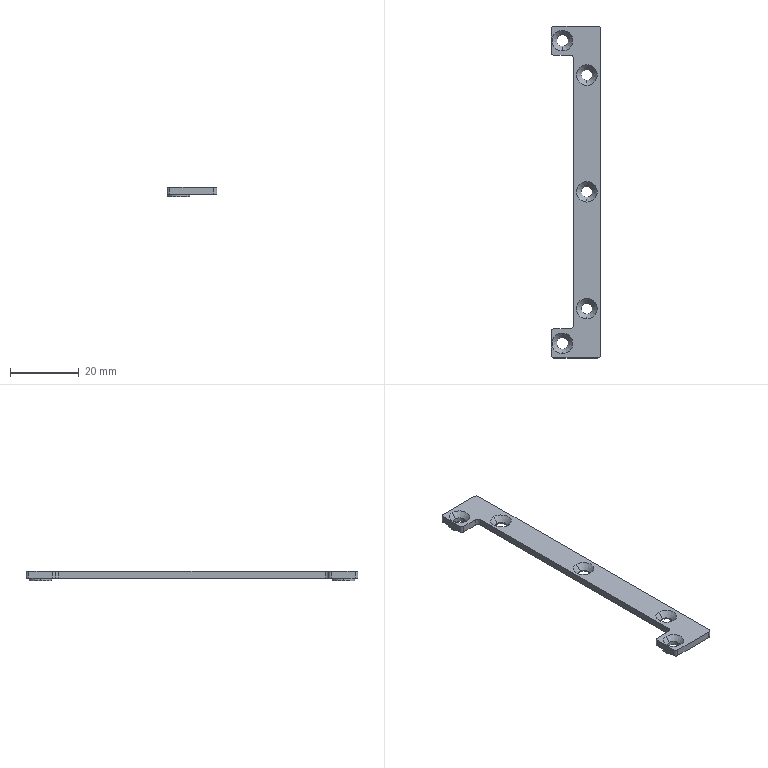NC program | NX | posted with a generic post | part box 14.52 x 96.5 x 2.7 mm
Whole program:
N10 G17 G21 G94 G90
(FLOOR_WALL , TOOL : D6)
N12 T06 M6
N14 G54
N16 G17 G0 G90 X57.25 Y-10.257 S9500 M3
N18 G43 Z30. H6
N20 Z3.
N22 G94 G1 Z0. F1500.
N24 X54.25
N26 X-54.25
N28 Y-7.669
N30 X54.25
N32 Y-5.081
N34 X-54.25
N36 Y-2.493
N38 X54.25
N40 Y0.096
N42 X-54.25
N44 Y2.684
N46 X54.25
N48 Y5.272
N50 X-54.25
N52 Y7.86
N54 X54.25
N56 X57.25
N58 Z3.
N60 G0 Z30.
N62 M5
(DRILLING , TOOL : D6A45)
N64 T07 M6
N66 G54
N68 G17 G0 G90 X-44. Y-3.96 S5000 M3
N70 G43 Z30. H7
N72 G94 G81 G98 Z-3. F250. R3.
N74 X-34. Y3.15
N76 X-0.05
N78 X33.9
N80 X44. Y-3.96
N82 G80
N84 G0 X44. Y-3.96 Z30.
N86 M5
(CAVITY_MILL , TOOL : D4)
N88 T04 M6
N90 G54
N92 G17 G0 G90 X2.078 Y-13.057 S9500 M3
N94 G43 Z30. H4
N96 Z0.614
N98 G95 G1 Z-0.386 F1.579
N100 X0.866 Y-10.957
N102 G3 X0. Y-10.457 R1.
N104 G94 G1 X-51.248 F2500.
N106 G2 X-51.448 Y-10.265 R0.205
N108 G1 Y10.265
N110 G2 X-51.248 Y10.458 R0.205
N112 G1 X51.248
N114 G2 X51.447 Y10.265 R0.205
N116 G1 Y-10.265
N118 G2 X51.248 Y-10.457 R0.204
N120 G1 X0.
N122 Y-7.657
N124 X-37.304
N126 G3 X-37.09 Y-6.46 R3.46
N128 G1 Y-3.32
N130 X37.09
N132 Y-6.46
N134 G3 X37.304 Y-7.657 R3.46
N136 G1 X37.829 Y-7.464
N138 G2 X37.65 Y-6.46 R2.9
N140 G1 Y-2.76
N142 X-37.65
N144 Y-6.46
N146 G2 X-40.55 Y-9.36 R2.9
N148 G1 X-47.45
N150 G2 X-50.35 Y-6.46 R2.9
N152 G1 Y6.26
N154 G2 X-47.25 Y9.36 R3.1
N156 G1 X47.25
N158 G2 X50.35 Y6.26 R3.1
N160 G1 Y-6.46
N162 G2 X47.45 Y-9.36 R2.9
N164 G1 X40.55
N166 G2 X37.829 Y-7.464 R2.9
N168 G1 X37.304 Y-7.657
N170 X0.
N172 Y-5.857
N174 X-35.29
N176 Y-5.12
N178 X35.29
N180 Y-5.857
N182 X0.
N184 G3 X-0.866 Y-6.357 R1.
N186 G1 Z0.614
N188 G0 Z30.
N190 X2.078 Y-13.058
N192 Z0.229
N194 G95 G1 Z-0.771 F1.579
N196 X0.866 Y-10.958
N198 G3 X0. Y-10.458 R1.
N200 G94 G1 X-51.248 F2500.
N202 G2 X-51.448 Y-10.265 R0.205
N204 G1 Y10.265
N206 G2 X-51.248 Y10.458 R0.205
N208 G1 X51.248
N210 G2 X51.447 Y10.265 R0.205
N212 G1 Y-10.265
N214 G2 X51.248 Y-10.458 R0.204
N216 G1 X0.
N218 Y-7.658
N220 X-37.304
N222 G3 X-37.09 Y-6.46 R3.46
N224 G1 Y-3.32
N226 X37.09
N228 Y-6.46
N230 G3 X37.304 Y-7.658 R3.46
N232 G1 X37.829 Y-7.464
N234 G2 X37.65 Y-6.46 R2.9
N236 G1 Y-2.76
N238 X-37.65
N240 Y-6.46
N242 G2 X-40.55 Y-9.36 R2.9
N244 G1 X-47.45
N246 G2 X-50.35 Y-6.46 R2.9
N248 G1 Y6.26
N250 G2 X-47.25 Y9.36 R3.1
N252 G1 X47.25
N254 G2 X50.35 Y6.26 R3.1
N256 G1 Y-6.46
N258 G2 X47.45 Y-9.36 R2.9
N260 G1 X40.55
N262 G2 X37.829 Y-7.464 R2.9
N264 G1 X37.304 Y-7.658
N266 X0.
N268 Y-5.858
N270 X-35.29
N272 Y-5.12
N274 X35.29
N276 Y-5.858
N278 X0.
N280 G3 X-0.866 Y-6.358 R1.
N282 G1 Z0.229
N284 G0 X2.078 Y-13.058 Z-0.157
N286 G95 G1 Z-1.157 F1.579
N288 X0.866 Y-10.958
N290 G3 X0. Y-10.458 R1.
N292 G94 G1 X-51.248 F2500.
N294 G2 X-51.448 Y-10.264 R0.205
N296 G1 Y10.265
N298 G2 X-51.248 Y10.459 R0.206
N300 G1 X51.247
N302 G2 X51.448 Y10.265 R0.205
N304 G1 Y-10.265
N306 G2 X51.248 Y-10.458 R0.205
N308 G1 X0.
N310 Y-7.658
N312 X-37.304
N314 G3 X-37.09 Y-6.46 R3.46
N316 G1 Y-3.32
N318 X37.09
N320 Y-6.46
N322 G3 X37.304 Y-7.658 R3.46
N324 G1 X37.829 Y-7.464
N326 G2 X37.65 Y-6.46 R2.9
N328 G1 Y-2.76
N330 X-37.65
N332 Y-6.46
N334 G2 X-40.55 Y-9.36 R2.9
N336 G1 X-47.45
N338 G2 X-50.35 Y-6.46 R2.9
N340 G1 Y6.26
N342 G2 X-47.25 Y9.36 R3.1
N344 G1 X47.25
N346 G2 X50.35 Y6.26 R3.1
N348 G1 Y-6.46
N350 G2 X47.45 Y-9.36 R2.9
N352 G1 X40.55
N354 G2 X37.829 Y-7.464 R2.9
N356 G1 X37.304 Y-7.658
N358 X0.
N360 Y-5.858
N362 X-35.29
N364 Y-5.12
N366 X35.29
N368 Y-5.858
N370 X0.
N372 G3 X-0.866 Y-6.358 R1.
N374 G1 Z-0.157
N376 G0 X2.078 Y-13.058 Z-0.543
N378 G95 G1 Z-1.543 F1.579
N380 X0.866 Y-10.958
N382 G3 X0. Y-10.458 R1.
N384 G94 G1 X-51.248 F2500.
N386 G2 X-51.449 Y-10.264 R0.206
N388 G1 Y10.264
N390 G2 X-51.247 Y10.459 R0.207
N392 G1 X51.247
N394 G2 X51.448 Y10.265 R0.206
N396 G1 Y-10.265
N398 G2 X51.248 Y-10.458 R0.205
N400 G1 X0.
N402 Y-7.658
N404 X-37.304
N406 G3 X-37.09 Y-6.46 R3.46
N408 G1 Y-3.32
N410 X37.09
N412 Y-6.46
N414 G3 X37.304 Y-7.658 R3.46
N416 G1 X37.829 Y-7.464
N418 G2 X37.65 Y-6.46 R2.9
N420 G1 Y-2.76
N422 X-37.65
N424 Y-6.46
N426 G2 X-40.55 Y-9.36 R2.9
N428 G1 X-47.45
N430 G2 X-50.35 Y-6.46 R2.9
N432 G1 Y6.26
N434 G2 X-47.25 Y9.36 R3.1
N436 G1 X47.25
N438 G2 X50.35 Y6.26 R3.1
N440 G1 Y-6.46
N442 G2 X47.45 Y-9.36 R2.9
N444 G1 X40.55
N446 G2 X37.829 Y-7.464 R2.9
N448 G1 X37.304 Y-7.658
N450 X0.
N452 Y-5.858
N454 X-35.29
N456 Y-5.12
N458 X35.29
N460 Y-5.858
N462 X0.
N464 G3 X-0.866 Y-6.358 R1.
N466 G1 Z-0.543
N468 G0 X2.078 Y-13.058 Z-0.929
N470 G95 G1 Z-1.929 F1.579
N472 X0.866 Y-10.958
N474 G3 X0. Y-10.458 R1.
N476 G94 G1 X-51.248 F2500.
N478 G2 X-51.449 Y-10.264 R0.206
N480 G1 Y10.264
N482 G2 X-51.247 Y10.459 R0.207
N484 G1 X51.247
N486 G2 X51.448 Y10.265 R0.206
N488 G1 Y-10.265
N490 G2 X51.248 Y-10.458 R0.205
N492 G1 X0.
N494 Y-7.658
N496 X-37.304
N498 G3 X-37.09 Y-6.46 R3.46
N500 G1 Y-3.32
N502 X37.09
N504 Y-6.46
N506 G3 X37.304 Y-7.658 R3.46
N508 G1 X37.829 Y-7.464
N510 G2 X37.65 Y-6.46 R2.9
N512 G1 Y-2.76
N514 X-37.65
N516 Y-6.46
N518 G2 X-40.55 Y-9.36 R2.9
N520 G1 X-47.45
N522 G2 X-50.35 Y-6.46 R2.9
N524 G1 Y6.26
N526 G2 X-47.25 Y9.36 R3.1
N528 G1 X47.25
N530 G2 X50.35 Y6.26 R3.1
N532 G1 Y-6.46
N534 G2 X47.45 Y-9.36 R2.9
N536 G1 X40.55
N538 G2 X37.829 Y-7.464 R2.9
N540 G1 X37.304 Y-7.658
N542 X0.
N544 Y-5.858
N546 X-35.29
N548 Y-5.12
N550 X35.29
N552 Y-5.858
N554 X0.
N556 G3 X-0.866 Y-6.358 R1.
N558 G1 Z-0.929
N560 G0 X2.078 Y-13.058 Z-1.314
N562 G95 G1 Z-2.314 F1.579
N564 X0.866 Y-10.958
N566 G3 X0. Y-10.458 R1.
N568 G94 G1 X-51.248 F2500.
N570 G2 X-51.449 Y-10.264 R0.207
N572 G1 Y10.264
N574 G2 X-51.247 Y10.46 R0.208
N576 G1 X51.247
N578 G2 X51.448 Y10.265 R0.207
N580 G1 Y-10.264
N582 G2 X51.248 Y-10.458 R0.206
N584 G1 X0.
N586 Y-7.658
N588 X-37.304
N590 G3 X-37.09 Y-6.46 R3.46
N592 G1 Y-3.32
N594 X37.09
N596 Y-6.46
N598 G3 X37.304 Y-7.658 R3.46
N600 G1 X37.829 Y-7.464
N602 G2 X37.65 Y-6.46 R2.9
N604 G1 Y-2.76
N606 X-37.65
N608 Y-6.46
N610 G2 X-40.55 Y-9.36 R2.9
N612 G1 X-47.45
N614 G2 X-50.35 Y-6.46 R2.9
N616 G1 Y6.26
N618 G2 X-47.25 Y9.36 R3.1
N620 G1 X47.25
N622 G2 X50.35 Y6.26 R3.1
N624 G1 Y-6.46
N626 G2 X47.45 Y-9.36 R2.9
N628 G1 X40.55
N630 G2 X37.829 Y-7.464 R2.9
N632 G1 X37.304 Y-7.658
N634 X0.
N636 Y-5.858
N638 X-35.29
N640 Y-5.12
N642 X35.29
N644 Y-5.858
N646 X0.
N648 G3 X-0.866 Y-6.358 R1.
N650 G1 Z-1.314
N652 G0 X2.078 Y-13.059 Z-1.7
N654 G95 G1 Z-2.7 F1.579
N656 X0.866 Y-10.959
N658 G3 X0. Y-10.459 R1.
N660 G94 G1 X-51.248 F2500.
N662 G2 X-51.45 Y-10.264 R0.207
N664 G1 Y10.264
N666 G2 X-51.247 Y10.46 R0.208
N668 G1 X51.247
N670 G2 X51.448 Y10.265 R0.207
N672 G1 Y-10.264
N674 G2 X51.248 Y-10.459 R0.206
N676 G1 X0.
N678 Y-7.659
N680 X-37.304
N682 G3 X-37.09 Y-6.46 R3.46
N684 G1 Y-3.32
N686 X37.09
N688 Y-6.46
N690 G3 X37.304 Y-7.659 R3.46
N692 G1 X37.83 Y-7.465
N694 G2 X37.65 Y-6.46 R2.9
N696 G1 Y-2.76
N698 X-37.65
N700 Y-6.46
N702 G2 X-40.55 Y-9.36 R2.9
N704 G1 X-47.45
N706 G2 X-50.35 Y-6.46 R2.9
N708 G1 Y6.26
N710 G2 X-47.25 Y9.36 R3.1
N712 G1 X47.25
N714 G2 X50.35 Y6.26 R3.1
N716 G1 Y-6.46
N718 G2 X47.45 Y-9.36 R2.9
N720 G1 X40.55
N722 G2 X37.83 Y-7.465 R2.9
N724 G1 X37.304 Y-7.659
N726 X0.
N728 Y-5.859
N730 X-35.29
N732 Y-5.12
N734 X35.29
N736 Y-5.859
N738 X0.
N740 G3 X-0.866 Y-6.359 R1.
N742 G1 Z-1.7
N744 G0 Z30.
(CAVITY_MILL_COPY , TOOL : D4)
N746 X-48.217 Y9.935
N748 Z-1.7
N750 G95 G1 Z-2.7 F1.579
N752 X-48.116 Y9.76
N754 G3 X-47.25 Y9.26 R1.
N756 G94 G1 X47.25 F1200.
N758 G2 X50.25 Y6.26 R3.
N760 G1 Y-6.46
N762 G2 X47.45 Y-9.26 R2.8
N764 G1 X40.55
N766 G2 X37.75 Y-6.46 R2.8
N768 G1 Y-2.66
N770 X-37.75
N772 Y-6.46
N774 G2 X-40.55 Y-9.26 R2.8
N776 G1 X-47.45
N778 G2 X-50.25 Y-6.46 R2.8
N780 G1 Y6.26
N782 G2 X-47.25 Y9.26 R3.
N784 G3 X-46.384 Y9.76 R1.
N786 G1 X-46.211 Y10.06
N788 Z-1.7
N790 G0 Z30.
N792 M5
(CAVITY_MILL_COPY_1 , TOOL : D2)
N794 T02 M6
N796 G54
N798 G17 G0 G90 X38.35 Y-3.759 S9500 M3
N800 G43 Z30. H2
N802 Z0.807
N804 G95 G1 Z-0.193 F1.579
N806 G3 X38.75 Y-2.959 R1.
N808 G94 G1 Y-1.66 F1200.
N810 X37.451
N812 G3 X36.651 Y-2.06 R1.
N814 G1 Z0.807
N816 G0 Z30.
N818 X38.35 Y-3.759
N820 Z0.614
N822 G95 G1 Z-0.386 F1.579
N824 G3 X38.75 Y-2.959 R1.
N826 G94 G1 Y-1.66 F1200.
N828 X37.451
N830 G3 X36.651 Y-2.06 R1.
N832 G1 Z0.614
N834 G0 Z30.
N836 X38.35 Y-3.759
N838 Z0.421
N840 G95 G1 Z-0.579 F1.579
N842 G3 X38.75 Y-2.959 R1.
N844 G94 G1 Y-1.66 F1200.
N846 X37.451
N848 G3 X36.651 Y-2.06 R1.
N850 G1 Z0.421
N852 G0 Z30.
N854 X38.35 Y-3.759
N856 Z0.229
N858 G95 G1 Z-0.771 F1.579
N860 G3 X38.75 Y-2.959 R1.
N862 G94 G1 Y-1.66 F1200.
N864 X37.451
N866 G3 X36.651 Y-2.06 R1.
N868 G1 Z0.229
N870 G0 Z30.
N872 X38.35 Y-3.759
N874 Z0.036
N876 G95 G1 Z-0.964 F1.579
N878 G3 X38.75 Y-2.959 R1.
N880 G94 G1 Y-1.66 F1200.
N882 X37.451
N884 G3 X36.651 Y-2.06 R1.
N886 G1 Z0.036
N888 G0 X38.35 Y-3.759 Z-0.157
N890 G95 G1 Z-1.157 F1.579
N892 G3 X38.75 Y-2.959 R1.
N894 G94 G1 Y-1.66 F1200.
N896 X37.451
N898 G3 X36.651 Y-2.06 R1.
N900 G1 Z-0.157
N902 G0 X38.35 Y-3.759 Z-0.35
N904 G95 G1 Z-1.35 F1.579
N906 G3 X38.75 Y-2.959 R1.
N908 G94 G1 Y-1.66 F1200.
N910 X37.451
N912 G3 X36.651 Y-2.06 R1.
N914 G1 Z-0.35
N916 G0 X38.35 Y-3.759 Z-0.543
N918 G95 G1 Z-1.543 F1.579
N920 G3 X38.75 Y-2.959 R1.
N922 G94 G1 Y-1.66 F1200.
N924 X37.451
N926 G3 X36.651 Y-2.06 R1.
N928 G1 Z-0.543
N930 G0 X38.35 Y-3.759 Z-0.736
N932 G95 G1 Z-1.736 F1.579
N934 G3 X38.75 Y-2.959 R1.
N936 G94 G1 Y-1.66 F1200.
N938 X37.451
N940 G3 X36.651 Y-2.06 R1.
N942 G1 Z-0.736
N944 G0 X38.35 Y-3.759 Z-0.929
N946 G95 G1 Z-1.929 F1.579
N948 G3 X38.75 Y-2.959 R1.
N950 G94 G1 Y-1.66 F1200.
N952 X37.451
N954 G3 X36.651 Y-2.06 R1.
N956 G1 Z-0.929
N958 G0 X38.35 Y-3.767 Z-1.121
N960 G95 G1 Z-2.121 F1.579
N962 G3 X38.75 Y-2.967 R1.
N964 G94 G1 Y-1.66 F1200.
N966 X37.45
N968 G3 X36.65 Y-2.06 R1.
N970 G1 Z-1.121
N972 G0 X38.35 Y-3.767 Z-1.314
N974 G95 G1 Z-2.314 F1.579
N976 G3 X38.75 Y-2.967 R1.
N978 G94 G1 Y-1.66 F1200.
N980 X37.45
N982 G3 X36.65 Y-2.06 R1.
N984 G1 Z-1.314
N986 G0 X38.35 Y-3.767 Z-1.507
N988 G95 G1 Z-2.507 F1.579
N990 G3 X38.75 Y-2.967 R1.
N992 G94 G1 Y-1.66 F1200.
N994 X37.45
N996 G3 X36.65 Y-2.06 R1.
N998 G1 Z-1.507
N1000 G0 X38.35 Y-3.767 Z-1.7
N1002 G95 G1 Z-2.7 F1.579
N1004 G3 X38.75 Y-2.967 R1.
N1006 G94 G1 Y-1.66 F1200.
N1008 X37.45
N1010 G3 X36.65 Y-2.06 R1.
N1012 G1 Z-1.7
N1014 G0 Z30.
N1016 X-36.651
N1018 Z0.807
N1020 G95 G1 Z-0.193 F1.579
N1022 G3 X-37.451 Y-1.66 R1.
N1024 G94 G1 X-38.75 F1200.
N1026 Y-2.959
N1028 G3 X-38.35 Y-3.759 R1.
N1030 G1 Z0.807
N1032 G0 Z30.
N1034 X-36.651 Y-2.06
N1036 Z0.614
N1038 G95 G1 Z-0.386 F1.579
N1040 G3 X-37.451 Y-1.66 R1.
N1042 G94 G1 X-38.75 F1200.
N1044 Y-2.959
N1046 G3 X-38.35 Y-3.759 R1.
N1048 G1 Z0.614
N1050 G0 Z30.
N1052 X-36.651 Y-2.06
N1054 Z0.421
N1056 G95 G1 Z-0.579 F1.579
N1058 G3 X-37.451 Y-1.66 R1.
N1060 G94 G1 X-38.75 F1200.
N1062 Y-2.959
N1064 G3 X-38.35 Y-3.759 R1.
N1066 G1 Z0.421
N1068 G0 Z30.
N1070 X-36.651 Y-2.06
N1072 Z0.229
N1074 G95 G1 Z-0.771 F1.579
N1076 G3 X-37.451 Y-1.66 R1.
N1078 G94 G1 X-38.75 F1200.
N1080 Y-2.959
N1082 G3 X-38.35 Y-3.759 R1.
N1084 G1 Z0.229
N1086 G0 Z30.
N1088 X-36.651 Y-2.06
N1090 Z0.036
N1092 G95 G1 Z-0.964 F1.579
N1094 G3 X-37.451 Y-1.66 R1.
N1096 G94 G1 X-38.75 F1200.
N1098 Y-2.959
N1100 G3 X-38.35 Y-3.759 R1.
N1102 G1 Z0.036
N1104 G0 X-36.651 Y-2.06 Z-0.157
N1106 G95 G1 Z-1.157 F1.579
N1108 G3 X-37.451 Y-1.66 R1.
N1110 G94 G1 X-38.75 F1200.
N1112 Y-2.959
N1114 G3 X-38.35 Y-3.759 R1.
N1116 G1 Z-0.157
N1118 G0 X-36.651 Y-2.06 Z-0.35
N1120 G95 G1 Z-1.35 F1.579
N1122 G3 X-37.451 Y-1.66 R1.
N1124 G94 G1 X-38.75 F1200.
N1126 Y-2.959
N1128 G3 X-38.35 Y-3.759 R1.
N1130 G1 Z-0.35
N1132 G0 X-36.651 Y-2.06 Z-0.543
N1134 G95 G1 Z-1.543 F1.579
N1136 G3 X-37.451 Y-1.66 R1.
N1138 G94 G1 X-38.75 F1200.
N1140 Y-2.959
N1142 G3 X-38.35 Y-3.759 R1.
N1144 G1 Z-0.543
N1146 G0 X-36.651 Y-2.06 Z-0.736
N1148 G95 G1 Z-1.736 F1.579
N1150 G3 X-37.451 Y-1.66 R1.
N1152 G94 G1 X-38.75 F1200.
N1154 Y-2.959
N1156 G3 X-38.35 Y-3.759 R1.
N1158 G1 Z-0.736
N1160 G0 X-36.651 Y-2.06 Z-0.929
N1162 G95 G1 Z-1.929 F1.579
N1164 G3 X-37.451 Y-1.66 R1.
N1166 G94 G1 X-38.75 F1200.
N1168 Y-2.959
N1170 G3 X-38.35 Y-3.759 R1.
N1172 G1 Z-0.929
N1174 G0 X-36.658 Y-2.06 Z-1.121
N1176 G95 G1 Z-2.121 F1.579
N1178 G3 X-37.458 Y-1.66 R1.
N1180 G94 G1 X-38.75 F1200.
N1182 Y-2.951
N1184 G3 X-38.35 Y-3.751 R1.
N1186 G1 Z-1.121
N1188 G0 X-36.658 Y-2.06 Z-1.314
N1190 G95 G1 Z-2.314 F1.579
N1192 G3 X-37.458 Y-1.66 R1.
N1194 G94 G1 X-38.75 F1200.
N1196 Y-2.951
N1198 G3 X-38.35 Y-3.751 R1.
N1200 G1 Z-1.314
N1202 G0 X-36.658 Y-2.06 Z-1.507
N1204 G95 G1 Z-2.507 F1.579
N1206 G3 X-37.458 Y-1.66 R1.
N1208 G94 G1 X-38.75 F1200.
N1210 Y-2.951
N1212 G3 X-38.35 Y-3.751 R1.
N1214 G1 Z-1.507
N1216 G0 X-36.658 Y-2.06 Z-1.7
N1218 G95 G1 Z-2.7 F1.579
N1220 G3 X-37.458 Y-1.66 R1.
N1222 G94 G1 X-38.75 F1200.
N1224 Y-2.951
N1226 G3 X-38.35 Y-3.751 R1.
N1228 G1 Z-1.7
N1230 G0 Z30.
(HOLE_MILLING , TOOL : D2)
N1232 X-44. Y-3.96
N1234 Z0.5
N1236 G3 X-43.65 Y-3.61 R0.35 F1250.
N1238 X-44. Y-3.26 R0.35
N1240 X-44. Y-3.26 Z0.3 I0. J-0.7
N1242 X-44. Y-3.26 Z0.1 I0. J-0.7
N1244 X-44. Y-3.26 Z-0.1 I0. J-0.7
N1246 X-44. Y-3.26 Z-0.3 I0. J-0.7
N1248 X-44. Y-3.26 Z-0.5 I0. J-0.7
N1250 X-44. Y-3.26 Z-0.7 I0. J-0.7
N1252 X-44. Y-3.26 Z-0.9 I0. J-0.7
N1254 X-44. Y-3.26 Z-1.1 I0. J-0.7
N1256 X-44. Y-3.26 Z-1.3 I0. J-0.7
N1258 X-44. Y-3.26 Z-1.5 I0. J-0.7
N1260 X-44. Y-3.26 Z-1.7 I0. J-0.7
N1262 X-44. Y-3.26 Z-1.9 I0. J-0.7
N1264 X-44. Y-3.26 Z-2.1 I0. J-0.7
N1266 X-44. Y-3.26 Z-2.3 I0. J-0.7
N1268 X-44. Y-3.26 Z-2.5 I0. J-0.7
N1270 X-44. Y-3.26 Z-2.7 I0. J-0.7
N1272 X-44.7 Y-3.96 R0.7
N1274 X-44. Y-3.26 R-0.7
N1276 X-44.35 Y-3.61 R0.35
N1278 X-44. Y-3.96 R0.35
N1280 G0 Z30.
N1282 X-34. Y3.15
N1284 Z0.5
N1286 G3 X-33.7 Y3.45 R0.3
N1288 X-34. Y3.75 R0.3
N1290 X-34. Y3.75 Z0.3 I0. J-0.6
N1292 X-34. Y3.75 Z0.1 I0. J-0.6
N1294 X-34. Y3.75 Z-0.1 I0. J-0.6
N1296 X-34. Y3.75 Z-0.3 I0. J-0.6
N1298 X-34. Y3.75 Z-0.5 I0. J-0.6
N1300 X-34. Y3.75 Z-0.7 I0. J-0.6
N1302 X-34. Y3.75 Z-0.9 I0. J-0.6
N1304 X-34. Y3.75 Z-1.1 I0. J-0.6
N1306 X-34. Y3.75 Z-1.3 I0. J-0.6
N1308 X-34. Y3.75 Z-1.5 I0. J-0.6
N1310 X-34. Y3.75 Z-1.7 I0. J-0.6
N1312 X-34. Y3.75 Z-1.9 I0. J-0.6
N1314 X-34. Y2.55 Z-2. I0. J-0.6
N1316 X-33.4 Y3.15 R0.6
N1318 X-34. Y2.55 R-0.6
N1320 X-33.7 Y2.85 R0.3
N1322 X-34. Y3.15 R0.3
N1324 G0 Z30.
N1326 X-0.05
N1328 Z0.5
N1330 G3 X0.25 Y3.45 R0.3
N1332 X-0.05 Y3.75 R0.3
N1334 X-0.05 Y3.75 Z0.3 I0. J-0.6
N1336 X-0.05 Y3.75 Z0.1 I0. J-0.6
N1338 X-0.05 Y3.75 Z-0.1 I0. J-0.6
N1340 X-0.05 Y3.75 Z-0.3 I0. J-0.6
N1342 X-0.05 Y3.75 Z-0.5 I0. J-0.6
N1344 X-0.05 Y3.75 Z-0.7 I0. J-0.6
N1346 X-0.05 Y3.75 Z-0.9 I0. J-0.6
N1348 X-0.05 Y3.75 Z-1.1 I0. J-0.6
N1350 X-0.05 Y3.75 Z-1.3 I0. J-0.6
N1352 X-0.05 Y3.75 Z-1.5 I0. J-0.6
N1354 X-0.05 Y3.75 Z-1.7 I0. J-0.6
N1356 X-0.05 Y3.75 Z-1.9 I0. J-0.6
N1358 X-0.05 Y2.55 Z-2. I0. J-0.6
N1360 X0.55 Y3.15 R0.6
N1362 X-0.05 Y2.55 R-0.6
N1364 X0.25 Y2.85 R0.3
N1366 X-0.05 Y3.15 R0.3
N1368 G0 Z30.
N1370 X33.9
N1372 Z0.5
N1374 G3 X34.2 Y3.45 R0.3
N1376 X33.9 Y3.75 R0.3
N1378 X33.9 Y3.75 Z0.3 I0. J-0.6
N1380 X33.9 Y3.75 Z0.1 I0. J-0.6
N1382 X33.9 Y3.75 Z-0.1 I0. J-0.6
N1384 X33.9 Y3.75 Z-0.3 I0. J-0.6
N1386 X33.9 Y3.75 Z-0.5 I0. J-0.6
N1388 X33.9 Y3.75 Z-0.7 I0. J-0.6
N1390 X33.9 Y3.75 Z-0.9 I0. J-0.6
N1392 X33.9 Y3.75 Z-1.1 I0. J-0.6
N1394 X33.9 Y3.75 Z-1.3 I0. J-0.6
N1396 X33.9 Y3.75 Z-1.5 I0. J-0.6
N1398 X33.9 Y3.75 Z-1.7 I0. J-0.6
N1400 X33.9 Y3.75 Z-1.9 I0. J-0.6
N1402 X33.9 Y2.55 Z-2. I0. J-0.6
N1404 X34.5 Y3.15 R0.6
N1406 X33.9 Y2.55 R-0.6
N1408 X34.2 Y2.85 R0.3
N1410 X33.9 Y3.15 R0.3
N1412 G0 Z30.
N1414 X44. Y-3.96
N1416 Z0.5
N1418 G3 X44.35 Y-3.61 R0.35
N1420 X44. Y-3.26 R0.35
N1422 X44. Y-3.26 Z0.3 I0. J-0.7
N1424 X44. Y-3.26 Z0.1 I0. J-0.7
N1426 X44. Y-3.26 Z-0.1 I0. J-0.7
N1428 X44. Y-3.26 Z-0.3 I0. J-0.7
N1430 X44. Y-3.26 Z-0.5 I0. J-0.7
N1432 X44. Y-3.26 Z-0.7 I0. J-0.7
N1434 X44. Y-3.26 Z-0.9 I0. J-0.7
N1436 X44. Y-3.26 Z-1.1 I0. J-0.7
N1438 X44. Y-3.26 Z-1.3 I0. J-0.7
N1440 X44. Y-3.26 Z-1.5 I0. J-0.7
N1442 X44. Y-3.26 Z-1.7 I0. J-0.7
N1444 X44. Y-3.26 Z-1.9 I0. J-0.7
N1446 X44. Y-3.26 Z-2.1 I0. J-0.7
N1448 X44. Y-3.26 Z-2.3 I0. J-0.7
N1450 X44. Y-3.26 Z-2.5 I0. J-0.7
N1452 X44. Y-3.26 Z-2.7 I0. J-0.7
N1454 X43.3 Y-3.96 R0.7
N1456 X44. Y-3.26 R-0.7
N1458 X43.65 Y-3.61 R0.35
N1460 X44. Y-3.96 R0.35
N1462 G0 Z30.
N1464 M5
(PLANAR_MILL , TOOL : D6A45)
N1466 T07 M6
N1468 G54
N1470 G17 G0 G90 X-39.414 Y-9.128 S9500 M3
N1472 G43 Z30. H7
N1474 Z0.5
N1476 G94 G1 Z-1. F1250.
N1478 X-39.684 Y-8.66
N1480 G3 X-40.55 Y-8.16 R1.
N1482 G1 X-47.45
N1484 G2 X-49.15 Y-6.46 R1.7
N1486 G1 Y6.26
N1488 G2 X-47.25 Y8.16 R1.9
N1490 G1 X47.25
N1492 G2 X49.15 Y6.26 R1.9
N1494 G1 Y-6.46
N1496 G2 X47.45 Y-8.16 R1.7
N1498 G1 X40.55
N1500 G2 X38.85 Y-6.46 R1.7
N1502 G1 Y-1.66
N1504 X38.863 Y-1.595
N1506 X38.815 Y-1.547
N1508 X38.75 Y-1.56
N1510 X-38.75
N1512 X-38.815 Y-1.547
N1514 X-38.863 Y-1.595
N1516 X-38.85 Y-1.66
N1518 Y-6.46
N1520 G2 X-40.55 Y-8.16 R1.7
N1522 G3 X-41.416 Y-8.66 R1.
N1524 G1 X-41.82 Y-9.36
N1526 Z0.5
N1528 G0 Z30.
N1530 M5
N1532 M2